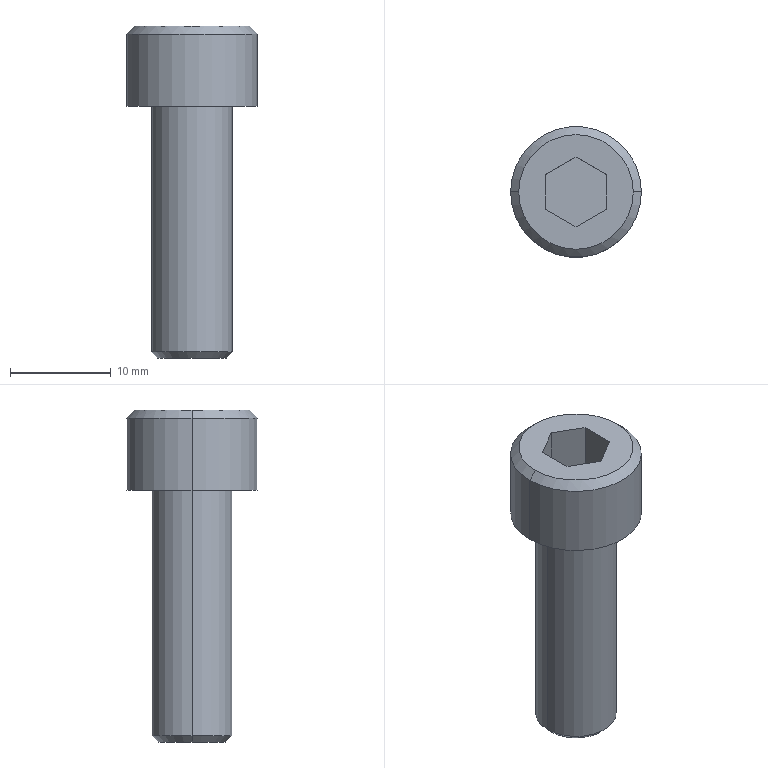Part | Creo | 1 solid | 18 faces | box 13 x 13 x 33 mm | volume 2152 mm3 | plane 10 | cylinder 4 | cone 4 | commonest cylinder face diameters 8 x2 13 x2
STEP:
#1=CARTESIAN_POINT('',(-183.5,-117.908,-52.5));
#2=VERTEX_POINT('',#1);
#3=CARTESIAN_POINT('',(-196.5,-117.908,-52.5));
#4=VERTEX_POINT('',#3);
#5=CARTESIAN_POINT('',(-190.,-117.908,-52.5));
#6=DIRECTION('',(0.,0.,-1.));
#7=DIRECTION('',(1.,0.,0.));
#8=AXIS2_PLACEMENT_3D('',#5,#6,#7);
#9=CIRCLE('',#8,6.5);
#10=EDGE_CURVE('',#2,#4,#9,.T.);
#11=ORIENTED_EDGE('',*,*,#10,.F.);
#12=CARTESIAN_POINT('',(-190.,-117.908,-52.5));
#13=DIRECTION('',(0.,0.,-1.));
#14=DIRECTION('',(-1.,0.,0.));
#15=AXIS2_PLACEMENT_3D('',#12,#13,#14);
#16=CIRCLE('',#15,6.5);
#17=EDGE_CURVE('',#4,#2,#16,.T.);
#18=ORIENTED_EDGE('',*,*,#17,.F.);
#19=EDGE_LOOP('',(#11,#18));
#20=FACE_OUTER_BOUND('',#19,.F.);
#21=CARTESIAN_POINT('',(-194.,-117.908,-52.5));
#22=VERTEX_POINT('',#21);
#23=CARTESIAN_POINT('',(-186.,-117.908,-52.5));
#24=VERTEX_POINT('',#23);
#25=CARTESIAN_POINT('',(-190.,-117.908,-52.5));
#26=DIRECTION('',(0.,0.,1.));
#27=DIRECTION('',(-1.,0.,0.));
#28=AXIS2_PLACEMENT_3D('',#25,#26,#27);
#29=CIRCLE('',#28,4.);
#30=EDGE_CURVE('',#22,#24,#29,.T.);
#31=ORIENTED_EDGE('',*,*,#30,.F.);
#32=CARTESIAN_POINT('',(-190.,-117.908,-52.5));
#33=DIRECTION('',(0.,0.,1.));
#34=DIRECTION('',(1.,0.,0.));
#35=AXIS2_PLACEMENT_3D('',#32,#33,#34);
#36=CIRCLE('',#35,4.);
#37=EDGE_CURVE('',#24,#22,#36,.T.);
#38=ORIENTED_EDGE('',*,*,#37,.F.);
#39=EDGE_LOOP('',(#31,#38));
#40=FACE_BOUND('',#39,.F.);
#41=CARTESIAN_POINT('',(-190.,-117.908,-52.5));
#42=DIRECTION('',(0.,0.,-1.));
#43=DIRECTION('',(-1.,0.,0.));
#44=AXIS2_PLACEMENT_3D('',#41,#42,#43);
#45=PLANE('',#44);
#46=ADVANCED_FACE('',(#20,#40),#45,.T.);
#47=CARTESIAN_POINT('',(-186.,-117.908,-76.9));
#48=VERTEX_POINT('',#47);
#49=CARTESIAN_POINT('',(-194.,-117.908,-76.9));
#50=VERTEX_POINT('',#49);
#51=CARTESIAN_POINT('',(-190.,-117.908,-76.9));
#52=DIRECTION('',(0.,0.,-1.));
#53=DIRECTION('',(1.,0.,0.));
#54=AXIS2_PLACEMENT_3D('',#51,#52,#53);
#55=CIRCLE('',#54,4.);
#56=EDGE_CURVE('',#48,#50,#55,.T.);
#57=ORIENTED_EDGE('',*,*,#56,.T.);
#58=CARTESIAN_POINT('',(-194.,-117.908,-52.5));
#59=DIRECTION('',(0.,0.,-1.));
#60=VECTOR('',#59,24.4);
#61=LINE('',#58,#60);
#62=EDGE_CURVE('',#22,#50,#61,.T.);
#63=ORIENTED_EDGE('',*,*,#62,.F.);
#64=ORIENTED_EDGE('',*,*,#30,.T.);
#65=CARTESIAN_POINT('',(-186.,-117.908,-52.5));
#66=DIRECTION('',(0.,0.,-1.));
#67=VECTOR('',#66,24.4);
#68=LINE('',#65,#67);
#69=EDGE_CURVE('',#24,#48,#68,.T.);
#70=ORIENTED_EDGE('',*,*,#69,.T.);
#71=EDGE_LOOP('',(#57,#63,#64,#70));
#72=FACE_OUTER_BOUND('',#71,.F.);
#73=CARTESIAN_POINT('',(-190.,-117.908,-43.5));
#74=DIRECTION('',(0.,0.,-1.));
#75=DIRECTION('',(-1.,0.,0.));
#76=AXIS2_PLACEMENT_3D('',#73,#74,#75);
#77=CYLINDRICAL_SURFACE('',#76,4.);
#78=ADVANCED_FACE('',(#72),#77,.T.);
#79=CARTESIAN_POINT('',(-186.6,-117.908,-77.5));
#80=VERTEX_POINT('',#79);
#81=CARTESIAN_POINT('',(-193.4,-117.908,-77.5));
#82=VERTEX_POINT('',#81);
#83=CARTESIAN_POINT('',(-190.,-117.908,-77.5));
#84=DIRECTION('',(0.,0.,-1.));
#85=DIRECTION('',(1.,0.,0.));
#86=AXIS2_PLACEMENT_3D('',#83,#84,#85);
#87=CIRCLE('',#86,3.4);
#88=EDGE_CURVE('',#80,#82,#87,.T.);
#89=ORIENTED_EDGE('',*,*,#88,.T.);
#90=CARTESIAN_POINT('',(-193.4,-117.908,-77.5));
#91=DIRECTION('',(-0.7071,0.,0.7071));
#92=VECTOR('',#91,0.8485);
#93=LINE('',#90,#92);
#94=EDGE_CURVE('',#82,#50,#93,.T.);
#95=ORIENTED_EDGE('',*,*,#94,.T.);
#96=ORIENTED_EDGE('',*,*,#56,.F.);
#97=CARTESIAN_POINT('',(-186.6,-117.908,-77.5));
#98=DIRECTION('',(0.7071,0.,0.7071));
#99=VECTOR('',#98,0.8485);
#100=LINE('',#97,#99);
#101=EDGE_CURVE('',#80,#48,#100,.T.);
#102=ORIENTED_EDGE('',*,*,#101,.F.);
#103=EDGE_LOOP('',(#89,#95,#96,#102));
#104=FACE_OUTER_BOUND('',#103,.F.);
#105=CARTESIAN_POINT('',(-190.,-117.908,-77.2));
#106=DIRECTION('',(0.,0.,1.));
#107=DIRECTION('',(1.,0.,0.));
#108=AXIS2_PLACEMENT_3D('',#105,#106,#107);
#109=CONICAL_SURFACE('',#108,3.7,45.);
#110=ADVANCED_FACE('',(#104),#109,.T.);
#111=CARTESIAN_POINT('',(-190.,-117.908,-77.5));
#112=DIRECTION('',(0.,0.,-1.));
#113=DIRECTION('',(-1.,0.,0.));
#114=AXIS2_PLACEMENT_3D('',#111,#112,#113);
#115=CIRCLE('',#114,3.4);
#116=EDGE_CURVE('',#82,#80,#115,.T.);
#117=ORIENTED_EDGE('',*,*,#116,.F.);
#118=ORIENTED_EDGE('',*,*,#88,.F.);
#119=EDGE_LOOP('',(#117,#118));
#120=FACE_OUTER_BOUND('',#119,.F.);
#121=CARTESIAN_POINT('',(-190.,-117.908,-77.5));
#122=DIRECTION('',(0.,0.,-1.));
#123=DIRECTION('',(-1.,0.,0.));
#124=AXIS2_PLACEMENT_3D('',#121,#122,#123);
#125=PLANE('',#124);
#126=ADVANCED_FACE('',(#120),#125,.T.);
#127=ORIENTED_EDGE('',*,*,#116,.T.);
#128=ORIENTED_EDGE('',*,*,#101,.T.);
#129=CARTESIAN_POINT('',(-190.,-117.908,-76.9));
#130=DIRECTION('',(0.,0.,-1.));
#131=DIRECTION('',(-1.,0.,0.));
#132=AXIS2_PLACEMENT_3D('',#129,#130,#131);
#133=CIRCLE('',#132,4.);
#134=EDGE_CURVE('',#50,#48,#133,.T.);
#135=ORIENTED_EDGE('',*,*,#134,.F.);
#136=ORIENTED_EDGE('',*,*,#94,.F.);
#137=EDGE_LOOP('',(#127,#128,#135,#136));
#138=FACE_OUTER_BOUND('',#137,.F.);
#139=CARTESIAN_POINT('',(-190.,-117.908,-77.2));
#140=DIRECTION('',(0.,0.,1.));
#141=DIRECTION('',(1.,0.,0.));
#142=AXIS2_PLACEMENT_3D('',#139,#140,#141);
#143=CONICAL_SURFACE('',#142,3.7,45.);
#144=ADVANCED_FACE('',(#138),#143,.T.);
#145=ORIENTED_EDGE('',*,*,#134,.T.);
#146=ORIENTED_EDGE('',*,*,#69,.F.);
#147=ORIENTED_EDGE('',*,*,#37,.T.);
#148=ORIENTED_EDGE('',*,*,#62,.T.);
#149=EDGE_LOOP('',(#145,#146,#147,#148));
#150=FACE_OUTER_BOUND('',#149,.F.);
#151=CARTESIAN_POINT('',(-190.,-117.908,-43.5));
#152=DIRECTION('',(0.,0.,-1.));
#153=DIRECTION('',(-1.,0.,0.));
#154=AXIS2_PLACEMENT_3D('',#151,#152,#153);
#155=CYLINDRICAL_SURFACE('',#154,4.);
#156=ADVANCED_FACE('',(#150),#155,.T.);
#157=CARTESIAN_POINT('',(-196.5,-117.908,-45.3));
#158=VERTEX_POINT('',#157);
#159=CARTESIAN_POINT('',(-183.5,-117.908,-45.3));
#160=VERTEX_POINT('',#159);
#161=CARTESIAN_POINT('',(-190.,-117.908,-45.3));
#162=DIRECTION('',(0.,0.,1.));
#163=DIRECTION('',(-1.,0.,0.));
#164=AXIS2_PLACEMENT_3D('',#161,#162,#163);
#165=CIRCLE('',#164,6.5);
#166=EDGE_CURVE('',#158,#160,#165,.T.);
#167=ORIENTED_EDGE('',*,*,#166,.T.);
#168=CARTESIAN_POINT('',(-183.5,-117.908,-45.3));
#169=DIRECTION('',(0.,0.,-1.));
#170=VECTOR('',#169,7.2);
#171=LINE('',#168,#170);
#172=EDGE_CURVE('',#160,#2,#171,.T.);
#173=ORIENTED_EDGE('',*,*,#172,.T.);
#174=ORIENTED_EDGE('',*,*,#10,.T.);
#175=CARTESIAN_POINT('',(-196.5,-117.908,-45.3));
#176=DIRECTION('',(0.,0.,-1.));
#177=VECTOR('',#176,7.2);
#178=LINE('',#175,#177);
#179=EDGE_CURVE('',#158,#4,#178,.T.);
#180=ORIENTED_EDGE('',*,*,#179,.F.);
#181=EDGE_LOOP('',(#167,#173,#174,#180));
#182=FACE_OUTER_BOUND('',#181,.F.);
#183=CARTESIAN_POINT('',(-190.,-117.908,-43.5));
#184=DIRECTION('',(0.,0.,-1.));
#185=DIRECTION('',(-1.,0.,0.));
#186=AXIS2_PLACEMENT_3D('',#183,#184,#185);
#187=CYLINDRICAL_SURFACE('',#186,6.5);
#188=ADVANCED_FACE('',(#182),#187,.T.);
#189=CARTESIAN_POINT('',(-195.7,-117.908,-44.5));
#190=VERTEX_POINT('',#189);
#191=CARTESIAN_POINT('',(-184.3,-117.908,-44.5));
#192=VERTEX_POINT('',#191);
#193=CARTESIAN_POINT('',(-190.,-117.908,-44.5));
#194=DIRECTION('',(0.,0.,1.));
#195=DIRECTION('',(-1.,0.,0.));
#196=AXIS2_PLACEMENT_3D('',#193,#194,#195);
#197=CIRCLE('',#196,5.7);
#198=EDGE_CURVE('',#190,#192,#197,.T.);
#199=ORIENTED_EDGE('',*,*,#198,.T.);
#200=CARTESIAN_POINT('',(-184.3,-117.908,-44.5));
#201=DIRECTION('',(0.7071,0.,-0.7071));
#202=VECTOR('',#201,1.131);
#203=LINE('',#200,#202);
#204=EDGE_CURVE('',#192,#160,#203,.T.);
#205=ORIENTED_EDGE('',*,*,#204,.T.);
#206=ORIENTED_EDGE('',*,*,#166,.F.);
#207=CARTESIAN_POINT('',(-195.7,-117.908,-44.5));
#208=DIRECTION('',(-0.7071,0.,-0.7071));
#209=VECTOR('',#208,1.131);
#210=LINE('',#207,#209);
#211=EDGE_CURVE('',#190,#158,#210,.T.);
#212=ORIENTED_EDGE('',*,*,#211,.F.);
#213=EDGE_LOOP('',(#199,#205,#206,#212));
#214=FACE_OUTER_BOUND('',#213,.F.);
#215=CARTESIAN_POINT('',(-190.,-117.908,-44.9));
#216=DIRECTION('',(0.,0.,-1.));
#217=DIRECTION('',(-1.,0.,0.));
#218=AXIS2_PLACEMENT_3D('',#215,#216,#217);
#219=CONICAL_SURFACE('',#218,6.1,45.);
#220=ADVANCED_FACE('',(#214),#219,.T.);
#221=ORIENTED_EDGE('',*,*,#198,.F.);
#222=CARTESIAN_POINT('',(-190.,-117.908,-44.5));
#223=DIRECTION('',(0.,0.,1.));
#224=DIRECTION('',(1.,0.,0.));
#225=AXIS2_PLACEMENT_3D('',#222,#223,#224);
#226=CIRCLE('',#225,5.7);
#227=EDGE_CURVE('',#192,#190,#226,.T.);
#228=ORIENTED_EDGE('',*,*,#227,.F.);
#229=EDGE_LOOP('',(#221,#228));
#230=FACE_OUTER_BOUND('',#229,.F.);
#231=CARTESIAN_POINT('',(-187.,-119.64,-44.5));
#232=VERTEX_POINT('',#231);
#233=CARTESIAN_POINT('',(-190.,-121.372,-44.5));
#234=VERTEX_POINT('',#233);
#235=CARTESIAN_POINT('',(-187.,-119.64,-44.5));
#236=DIRECTION('',(-0.866,-0.5,0.));
#237=VECTOR('',#236,3.464);
#238=LINE('',#235,#237);
#239=EDGE_CURVE('',#232,#234,#238,.T.);
#240=ORIENTED_EDGE('',*,*,#239,.F.);
#241=CARTESIAN_POINT('',(-187.,-116.176,-44.5));
#242=VERTEX_POINT('',#241);
#243=CARTESIAN_POINT('',(-187.,-116.176,-44.5));
#244=DIRECTION('',(0.,-1.,0.));
#245=VECTOR('',#244,3.464);
#246=LINE('',#243,#245);
#247=EDGE_CURVE('',#242,#232,#246,.T.);
#248=ORIENTED_EDGE('',*,*,#247,.F.);
#249=CARTESIAN_POINT('',(-190.,-114.444,-44.5));
#250=VERTEX_POINT('',#249);
#251=CARTESIAN_POINT('',(-190.,-114.444,-44.5));
#252=DIRECTION('',(0.866,-0.5,0.));
#253=VECTOR('',#252,3.464);
#254=LINE('',#251,#253);
#255=EDGE_CURVE('',#250,#242,#254,.T.);
#256=ORIENTED_EDGE('',*,*,#255,.F.);
#257=CARTESIAN_POINT('',(-193.,-116.176,-44.5));
#258=VERTEX_POINT('',#257);
#259=CARTESIAN_POINT('',(-193.,-116.176,-44.5));
#260=DIRECTION('',(0.866,0.5,0.));
#261=VECTOR('',#260,3.464);
#262=LINE('',#259,#261);
#263=EDGE_CURVE('',#258,#250,#262,.T.);
#264=ORIENTED_EDGE('',*,*,#263,.F.);
#265=CARTESIAN_POINT('',(-193.,-119.64,-44.5));
#266=VERTEX_POINT('',#265);
#267=CARTESIAN_POINT('',(-193.,-119.64,-44.5));
#268=DIRECTION('',(0.,1.,0.));
#269=VECTOR('',#268,3.464);
#270=LINE('',#267,#269);
#271=EDGE_CURVE('',#266,#258,#270,.T.);
#272=ORIENTED_EDGE('',*,*,#271,.F.);
#273=CARTESIAN_POINT('',(-190.,-121.372,-44.5));
#274=DIRECTION('',(-0.866,0.5,0.));
#275=VECTOR('',#274,3.464);
#276=LINE('',#273,#275);
#277=EDGE_CURVE('',#234,#266,#276,.T.);
#278=ORIENTED_EDGE('',*,*,#277,.F.);
#279=EDGE_LOOP('',(#240,#248,#256,#264,#272,#278));
#280=FACE_BOUND('',#279,.F.);
#281=CARTESIAN_POINT('',(-190.,-117.908,-44.5));
#282=DIRECTION('',(0.,0.,-1.));
#283=DIRECTION('',(-1.,0.,0.));
#284=AXIS2_PLACEMENT_3D('',#281,#282,#283);
#285=PLANE('',#284);
#286=ADVANCED_FACE('',(#230,#280),#285,.F.);
#287=ORIENTED_EDGE('',*,*,#227,.T.);
#288=ORIENTED_EDGE('',*,*,#211,.T.);
#289=CARTESIAN_POINT('',(-190.,-117.908,-45.3));
#290=DIRECTION('',(0.,0.,1.));
#291=DIRECTION('',(1.,0.,0.));
#292=AXIS2_PLACEMENT_3D('',#289,#290,#291);
#293=CIRCLE('',#292,6.5);
#294=EDGE_CURVE('',#160,#158,#293,.T.);
#295=ORIENTED_EDGE('',*,*,#294,.F.);
#296=ORIENTED_EDGE('',*,*,#204,.F.);
#297=EDGE_LOOP('',(#287,#288,#295,#296));
#298=FACE_OUTER_BOUND('',#297,.F.);
#299=CARTESIAN_POINT('',(-190.,-117.908,-44.9));
#300=DIRECTION('',(0.,0.,-1.));
#301=DIRECTION('',(-1.,0.,0.));
#302=AXIS2_PLACEMENT_3D('',#299,#300,#301);
#303=CONICAL_SURFACE('',#302,6.1,45.);
#304=ADVANCED_FACE('',(#298),#303,.T.);
#305=ORIENTED_EDGE('',*,*,#294,.T.);
#306=ORIENTED_EDGE('',*,*,#179,.T.);
#307=ORIENTED_EDGE('',*,*,#17,.T.);
#308=ORIENTED_EDGE('',*,*,#172,.F.);
#309=EDGE_LOOP('',(#305,#306,#307,#308));
#310=FACE_OUTER_BOUND('',#309,.F.);
#311=CARTESIAN_POINT('',(-190.,-117.908,-43.5));
#312=DIRECTION('',(0.,0.,-1.));
#313=DIRECTION('',(-1.,0.,0.));
#314=AXIS2_PLACEMENT_3D('',#311,#312,#313);
#315=CYLINDRICAL_SURFACE('',#314,6.5);
#316=ADVANCED_FACE('',(#310),#315,.T.);
#317=ORIENTED_EDGE('',*,*,#239,.T.);
#318=CARTESIAN_POINT('',(-190.,-121.372,-49.3));
#319=VERTEX_POINT('',#318);
#320=CARTESIAN_POINT('',(-190.,-121.372,-44.5));
#321=DIRECTION('',(0.,0.,-1.));
#322=VECTOR('',#321,4.8);
#323=LINE('',#320,#322);
#324=EDGE_CURVE('',#234,#319,#323,.T.);
#325=ORIENTED_EDGE('',*,*,#324,.T.);
#326=CARTESIAN_POINT('',(-187.,-119.64,-49.3));
#327=VERTEX_POINT('',#326);
#328=CARTESIAN_POINT('',(-190.,-121.372,-49.3));
#329=DIRECTION('',(0.866,0.5,0.));
#330=VECTOR('',#329,3.464);
#331=LINE('',#328,#330);
#332=EDGE_CURVE('',#319,#327,#331,.T.);
#333=ORIENTED_EDGE('',*,*,#332,.T.);
#334=CARTESIAN_POINT('',(-187.,-119.64,-44.5));
#335=DIRECTION('',(0.,0.,-1.));
#336=VECTOR('',#335,4.8);
#337=LINE('',#334,#336);
#338=EDGE_CURVE('',#232,#327,#337,.T.);
#339=ORIENTED_EDGE('',*,*,#338,.F.);
#340=EDGE_LOOP('',(#317,#325,#333,#339));
#341=FACE_OUTER_BOUND('',#340,.F.);
#342=CARTESIAN_POINT('',(-190.,-121.372,-49.3));
#343=DIRECTION('',(0.5,-0.866,0.));
#344=DIRECTION('',(0.866,0.5,0.));
#345=AXIS2_PLACEMENT_3D('',#342,#343,#344);
#346=PLANE('',#345);
#347=ADVANCED_FACE('',(#341),#346,.F.);
#348=ORIENTED_EDGE('',*,*,#277,.T.);
#349=CARTESIAN_POINT('',(-193.,-119.64,-49.3));
#350=VERTEX_POINT('',#349);
#351=CARTESIAN_POINT('',(-193.,-119.64,-44.5));
#352=DIRECTION('',(0.,0.,-1.));
#353=VECTOR('',#352,4.8);
#354=LINE('',#351,#353);
#355=EDGE_CURVE('',#266,#350,#354,.T.);
#356=ORIENTED_EDGE('',*,*,#355,.T.);
#357=CARTESIAN_POINT('',(-193.,-119.64,-49.3));
#358=DIRECTION('',(0.866,-0.5,0.));
#359=VECTOR('',#358,3.464);
#360=LINE('',#357,#359);
#361=EDGE_CURVE('',#350,#319,#360,.T.);
#362=ORIENTED_EDGE('',*,*,#361,.T.);
#363=ORIENTED_EDGE('',*,*,#324,.F.);
#364=EDGE_LOOP('',(#348,#356,#362,#363));
#365=FACE_OUTER_BOUND('',#364,.F.);
#366=CARTESIAN_POINT('',(-193.,-119.64,-49.3));
#367=DIRECTION('',(-0.5,-0.866,0.));
#368=DIRECTION('',(0.866,-0.5,0.));
#369=AXIS2_PLACEMENT_3D('',#366,#367,#368);
#370=PLANE('',#369);
#371=ADVANCED_FACE('',(#365),#370,.F.);
#372=ORIENTED_EDGE('',*,*,#271,.T.);
#373=CARTESIAN_POINT('',(-193.,-116.176,-49.3));
#374=VERTEX_POINT('',#373);
#375=CARTESIAN_POINT('',(-193.,-116.176,-44.5));
#376=DIRECTION('',(0.,0.,-1.));
#377=VECTOR('',#376,4.8);
#378=LINE('',#375,#377);
#379=EDGE_CURVE('',#258,#374,#378,.T.);
#380=ORIENTED_EDGE('',*,*,#379,.T.);
#381=CARTESIAN_POINT('',(-193.,-119.64,-49.3));
#382=DIRECTION('',(0.,1.,0.));
#383=VECTOR('',#382,3.464);
#384=LINE('',#381,#383);
#385=EDGE_CURVE('',#350,#374,#384,.T.);
#386=ORIENTED_EDGE('',*,*,#385,.F.);
#387=ORIENTED_EDGE('',*,*,#355,.F.);
#388=EDGE_LOOP('',(#372,#380,#386,#387));
#389=FACE_OUTER_BOUND('',#388,.F.);
#390=CARTESIAN_POINT('',(-193.,-116.176,-49.3));
#391=DIRECTION('',(-1.,0.,0.));
#392=DIRECTION('',(0.,0.,1.));
#393=AXIS2_PLACEMENT_3D('',#390,#391,#392);
#394=PLANE('',#393);
#395=ADVANCED_FACE('',(#389),#394,.F.);
#396=ORIENTED_EDGE('',*,*,#263,.T.);
#397=CARTESIAN_POINT('',(-190.,-114.444,-49.3));
#398=VERTEX_POINT('',#397);
#399=CARTESIAN_POINT('',(-190.,-114.444,-44.5));
#400=DIRECTION('',(0.,0.,-1.));
#401=VECTOR('',#400,4.8);
#402=LINE('',#399,#401);
#403=EDGE_CURVE('',#250,#398,#402,.T.);
#404=ORIENTED_EDGE('',*,*,#403,.T.);
#405=CARTESIAN_POINT('',(-190.,-114.444,-49.3));
#406=DIRECTION('',(-0.866,-0.5,0.));
#407=VECTOR('',#406,3.464);
#408=LINE('',#405,#407);
#409=EDGE_CURVE('',#398,#374,#408,.T.);
#410=ORIENTED_EDGE('',*,*,#409,.T.);
#411=ORIENTED_EDGE('',*,*,#379,.F.);
#412=EDGE_LOOP('',(#396,#404,#410,#411));
#413=FACE_OUTER_BOUND('',#412,.F.);
#414=CARTESIAN_POINT('',(-190.,-114.444,-49.3));
#415=DIRECTION('',(-0.5,0.866,0.));
#416=DIRECTION('',(-0.866,-0.5,0.));
#417=AXIS2_PLACEMENT_3D('',#414,#415,#416);
#418=PLANE('',#417);
#419=ADVANCED_FACE('',(#413),#418,.F.);
#420=ORIENTED_EDGE('',*,*,#255,.T.);
#421=CARTESIAN_POINT('',(-187.,-116.176,-49.3));
#422=VERTEX_POINT('',#421);
#423=CARTESIAN_POINT('',(-187.,-116.176,-44.5));
#424=DIRECTION('',(0.,0.,-1.));
#425=VECTOR('',#424,4.8);
#426=LINE('',#423,#425);
#427=EDGE_CURVE('',#242,#422,#426,.T.);
#428=ORIENTED_EDGE('',*,*,#427,.T.);
#429=CARTESIAN_POINT('',(-187.,-116.176,-49.3));
#430=DIRECTION('',(-0.866,0.5,0.));
#431=VECTOR('',#430,3.464);
#432=LINE('',#429,#431);
#433=EDGE_CURVE('',#422,#398,#432,.T.);
#434=ORIENTED_EDGE('',*,*,#433,.T.);
#435=ORIENTED_EDGE('',*,*,#403,.F.);
#436=EDGE_LOOP('',(#420,#428,#434,#435));
#437=FACE_OUTER_BOUND('',#436,.F.);
#438=CARTESIAN_POINT('',(-187.,-116.176,-49.3));
#439=DIRECTION('',(0.5,0.866,0.));
#440=DIRECTION('',(-0.866,0.5,0.));
#441=AXIS2_PLACEMENT_3D('',#438,#439,#440);
#442=PLANE('',#441);
#443=ADVANCED_FACE('',(#437),#442,.F.);
#444=ORIENTED_EDGE('',*,*,#247,.T.);
#445=ORIENTED_EDGE('',*,*,#338,.T.);
#446=CARTESIAN_POINT('',(-187.,-116.176,-49.3));
#447=DIRECTION('',(0.,-1.,0.));
#448=VECTOR('',#447,3.464);
#449=LINE('',#446,#448);
#450=EDGE_CURVE('',#422,#327,#449,.T.);
#451=ORIENTED_EDGE('',*,*,#450,.F.);
#452=ORIENTED_EDGE('',*,*,#427,.F.);
#453=EDGE_LOOP('',(#444,#445,#451,#452));
#454=FACE_OUTER_BOUND('',#453,.F.);
#455=CARTESIAN_POINT('',(-187.,-119.64,-49.3));
#456=DIRECTION('',(1.,0.,0.));
#457=DIRECTION('',(0.,0.,-1.));
#458=AXIS2_PLACEMENT_3D('',#455,#456,#457);
#459=PLANE('',#458);
#460=ADVANCED_FACE('',(#454),#459,.F.);
#461=ORIENTED_EDGE('',*,*,#361,.F.);
#462=ORIENTED_EDGE('',*,*,#385,.T.);
#463=ORIENTED_EDGE('',*,*,#409,.F.);
#464=ORIENTED_EDGE('',*,*,#433,.F.);
#465=ORIENTED_EDGE('',*,*,#450,.T.);
#466=ORIENTED_EDGE('',*,*,#332,.F.);
#467=EDGE_LOOP('',(#461,#462,#463,#464,#465,#466));
#468=FACE_OUTER_BOUND('',#467,.F.);
#469=CARTESIAN_POINT('',(-187.,-123.104,-49.3));
#470=DIRECTION('',(0.,0.,1.));
#471=DIRECTION('',(1.,0.,0.));
#472=AXIS2_PLACEMENT_3D('',#469,#470,#471);
#473=PLANE('',#472);
#474=ADVANCED_FACE('',(#468),#473,.T.);
#475=CLOSED_SHELL('',(#46,#78,#110,#126,#144,#156,#188,#220,#286,#304,#316,#347,#371,#395,#419,#443,#460,#474));
#476=MANIFOLD_SOLID_BREP('',#475);
#477=(LENGTH_UNIT()NAMED_UNIT(*)SI_UNIT(.MILLI.,.METRE.));
#478=UNCERTAINTY_MEASURE_WITH_UNIT(LENGTH_MEASURE(0.003778),#477,'','');
#479=(NAMED_UNIT(*)PLANE_ANGLE_UNIT()SI_UNIT($,.RADIAN.));
#480=PLANE_ANGLE_MEASURE_WITH_UNIT(PLANE_ANGLE_MEASURE(0.01745),#479);
#481=(CONVERSION_BASED_UNIT('DEGREE',#480)NAMED_UNIT(*)PLANE_ANGLE_UNIT());
#482=(NAMED_UNIT(*)SI_UNIT($,.STERADIAN.)SOLID_ANGLE_UNIT());
#483=(GEOMETRIC_REPRESENTATION_CONTEXT(3)GLOBAL_UNCERTAINTY_ASSIGNED_CONTEXT((#478))GLOBAL_UNIT_ASSIGNED_CONTEXT((#477,#481,#482))REPRESENTATION_CONTEXT('',''));
#484=ADVANCED_BREP_SHAPE_REPRESENTATION('',(#476),#483);